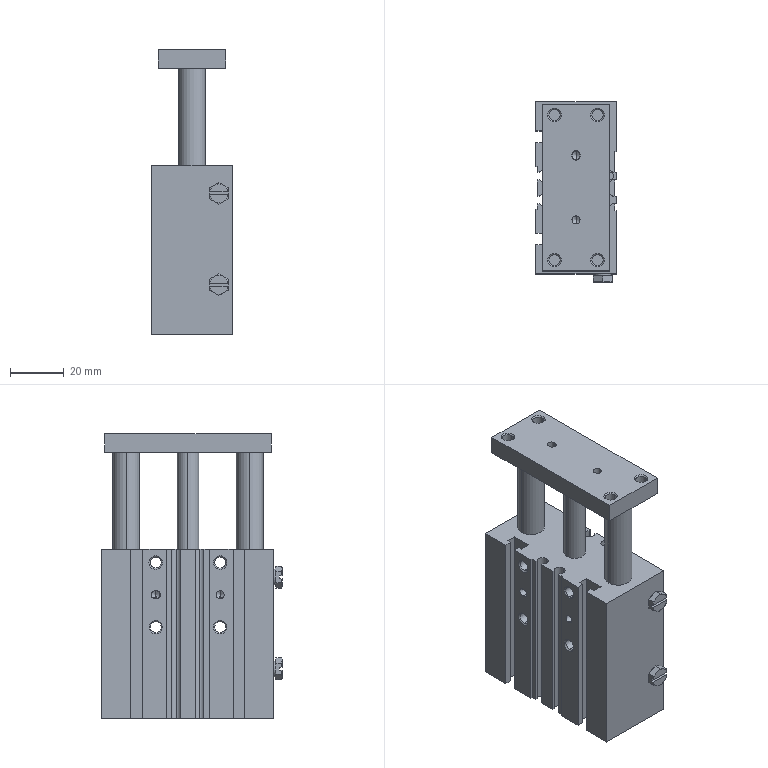Part | SolidWorks | features BaseBody 6 | 6 solids | 349 faces | box 30 x 67 x 106 mm | volume 115242 mm3 | plane 128 | cylinder 117 | cone 104 | commonest cylinder face diameters 4.134 x32 3 x18 8 x12 4.3 x8 10 x8 2.7 x6